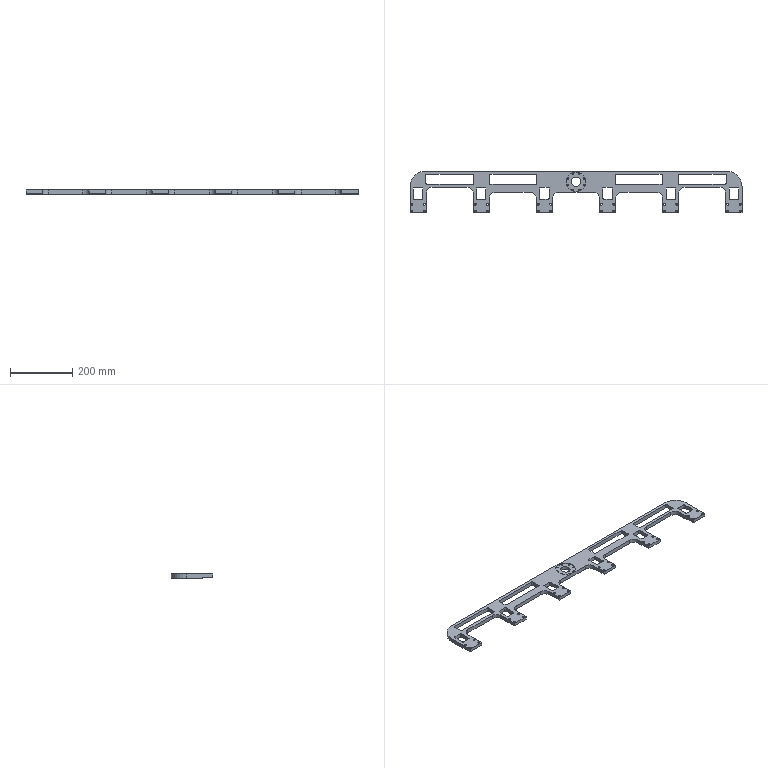NC program | NX | posted with a generic post | part box 1068 x 134 x 13 mm
Lines 1 to 1284 of 4175:
N10 G17 G21 G94 G90
(FLOOR_WALL_COPY_COPY , TOOL : D63)
N12 T01 M6
N14 G54
N16 G17 G0 G90 X572.5 Y-70.997 S6500 M3
N18 G43 Z30. H1
N20 Z4.
N22 G94 G1 Z1. F1500.
N24 X569.5
N26 X117.6
N28 Y-41.798
N30 X569.5
N32 Y-12.599
N34 X117.6
N36 Y16.601
N38 X569.5
N40 Y45.8
N42 X117.6
N44 Y74.999
N46 X569.5
N48 X572.5
N50 Z4.
N52 G0 Z30.
N54 Y-70.997
N56 Z3.
N58 G1 Z0.
N60 X569.5
N62 X117.6
N64 Y-41.798
N66 X569.5
N68 Y-12.599
N70 X117.6
N72 Y16.601
N74 X569.5
N76 Y45.8
N78 X117.6
N80 Y74.999
N82 X569.5
N84 X572.5
N86 Z3.
N88 G0 Z30.
N90 M5
(DRILLING_COPY_1_COPY , TOOL : D6A45)
N92 T07 M6
N94 G54
N96 G17 G0 G90 X284.8 Y-39.2 S5000 M3
N98 G43 Z30. H7
N100 G94 G81 G98 Z-1. F250. R3.
N102 Y-61.2
N104 X324.8
N106 Y-39.2
N108 X488.
N110 Y-61.2
N112 X528.
N114 Y-39.2
N116 G80
N118 G0 X528. Y-39.2 Z30.
N120 M5
(DRILLING_COPY_COPY_COPY_COPY , TOOL : 6.5ZT)
N122 T15 M6
N124 G54
N126 G17 G0 G90 X284.8 Y-39.2 S2000 M3
N128 G43 Z30. H15
N130 G94 G83 G98 Z-15.953 F250. Q2. R3.
N132 Y-61.2
N134 X324.8
N136 Y-39.2
N138 X488.
N140 Y-61.2
N142 X528.
N144 Y-39.2
N146 G80
N148 G0 X528. Y-39.2 Z30.
N150 M5
(ZLEVEL_PROFILE_COPY_3_COPY_1 , TOOL : D10)
N152 T10 M6
N154 G54
N156 G17 G0 G90 X115.002 Y75.6 S9500 M3
N158 G43 Z30. H10
N160 Z4.046
N162 G94 G1 Z-0.954 F1000.
N164 X116.734 Y72.6
N166 G3 X117.6 Y72.1 R1.
N168 G1 X484. F3500.
N170 G2 X539.1 Y17. R55.1
N172 G1 Y-67.
N174 G2 X534. Y-72.1 R5.1
N176 G1 X482.
N178 G2 X476.9 Y-67. R5.1
N180 G1 Y-5.
N182 G3 X462. Y9.9 R14.9
N184 G1 X350.8
N186 G3 X335.9 Y-5. R14.9
N188 G1 Y-67.
N190 G2 X330.8 Y-72.1 R5.1
N192 G1 X278.8
N194 G2 X273.7 Y-67. R5.1
N196 G1 Y-20.95
N198 G3 X258.8 Y-6.05 R14.9
N200 G1 X147.6
N202 G3 X132.7 Y-20.95 R14.9
N204 G1 Y-67.
N206 G2 X127.6 Y-72.1 R5.1
N208 G1 X117.6
N210 G3 X116.734 Y-72.6 R1.
N212 G1 X115.002 Y-75.6
N214 Z4.046
N216 G0 Z30.
N218 Z3.092
N220 G1 Z-1.908 F1000.
N222 X116.734 Y-72.6
N224 G2 X117.6 Y-72.1 R1.
N226 G1 X127.6 F3500.
N228 G3 X132.7 Y-67. R5.1
N230 G1 Y-20.95
N232 G2 X147.6 Y-6.05 R14.9
N234 G1 X258.8
N236 G2 X273.7 Y-20.95 R14.9
N238 G1 Y-67.
N240 G3 X278.8 Y-72.1 R5.1
N242 G1 X330.8
N244 G3 X335.9 Y-67. R5.1
N246 G1 Y-5.
N248 G2 X350.8 Y9.9 R14.9
N250 G1 X462.
N252 G2 X476.9 Y-5. R14.9
N254 G1 Y-67.
N256 G3 X482. Y-72.1 R5.1
N258 G1 X534.
N260 G3 X539.1 Y-67. R5.1
N262 G1 Y17.
N264 G3 X484. Y72.1 R55.1
N266 G1 X117.6
N268 G2 X116.734 Y72.6 R1.
N270 G1 X115.002 Y75.6
N272 Z3.092
N274 G0 Z30.
N276 Z2.138
N278 G1 Z-2.862 F1000.
N280 X116.734 Y72.6
N282 G3 X117.6 Y72.1 R1.
N284 G1 X484. F3500.
N286 G2 X539.1 Y17. R55.1
N288 G1 Y-67.
N290 G2 X534. Y-72.1 R5.1
N292 G1 X482.
N294 G2 X476.9 Y-67. R5.1
N296 G1 Y-5.
N298 G3 X462. Y9.9 R14.9
N300 G1 X350.8
N302 G3 X335.9 Y-5. R14.9
N304 G1 Y-67.
N306 G2 X330.8 Y-72.1 R5.1
N308 G1 X278.8
N310 G2 X273.7 Y-67. R5.1
N312 G1 Y-20.95
N314 G3 X258.8 Y-6.05 R14.9
N316 G1 X147.6
N318 G3 X132.7 Y-20.95 R14.9
N320 G1 Y-67.
N322 G2 X127.6 Y-72.1 R5.1
N324 G1 X117.6
N326 G3 X116.734 Y-72.6 R1.
N328 G1 X115.002 Y-75.6
N330 Z2.138
N332 G0 Z30.
N334 Z1.185
N336 G1 Z-3.815 F1000.
N338 X116.734 Y-72.6
N340 G2 X117.6 Y-72.1 R1.
N342 G1 X127.6 F3500.
N344 G3 X132.7 Y-67. R5.1
N346 G1 Y-20.95
N348 G2 X147.6 Y-6.05 R14.9
N350 G1 X258.8
N352 G2 X273.7 Y-20.95 R14.9
N354 G1 Y-67.
N356 G3 X278.8 Y-72.1 R5.1
N358 G1 X330.8
N360 G3 X335.9 Y-67. R5.1
N362 G1 Y-5.
N364 G2 X350.8 Y9.9 R14.9
N366 G1 X462.
N368 G2 X476.9 Y-5. R14.9
N370 G1 Y-67.
N372 G3 X482. Y-72.1 R5.1
N374 G1 X534.
N376 G3 X539.1 Y-67. R5.1
N378 G1 Y17.
N380 G3 X484. Y72.1 R55.1
N382 G1 X117.6
N384 G2 X116.734 Y72.6 R1.
N386 G1 X115.002 Y75.6
N388 Z1.185
N390 G0 Z30.
N392 Z0.231
N394 G1 Z-4.769 F1000.
N396 X116.734 Y72.6
N398 G3 X117.6 Y72.1 R1.
N400 G1 X484. F3500.
N402 G2 X539.1 Y17. R55.1
N404 G1 Y-67.
N406 G2 X534. Y-72.1 R5.1
N408 G1 X482.
N410 G2 X476.9 Y-67. R5.1
N412 G1 Y-5.
N414 G3 X462. Y9.9 R14.9
N416 G1 X350.8
N418 G3 X335.9 Y-5. R14.9
N420 G1 Y-67.
N422 G2 X330.8 Y-72.1 R5.1
N424 G1 X278.8
N426 G2 X273.7 Y-67. R5.1
N428 G1 Y-20.95
N430 G3 X258.8 Y-6.05 R14.9
N432 G1 X147.6
N434 G3 X132.7 Y-20.95 R14.9
N436 G1 Y-67.
N438 G2 X127.6 Y-72.1 R5.1
N440 G1 X117.6
N442 G3 X116.734 Y-72.6 R1.
N444 G1 X115.002 Y-75.6
N446 Z0.231
N448 G0 Z30.
N450 Z-0.723
N452 G1 Z-5.723 F1000.
N454 X116.734 Y-72.6
N456 G2 X117.6 Y-72.1 R1.
N458 G1 X127.6 F3500.
N460 G3 X132.7 Y-67. R5.1
N462 G1 Y-20.95
N464 G2 X147.6 Y-6.05 R14.9
N466 G1 X258.8
N468 G2 X273.7 Y-20.95 R14.9
N470 G1 Y-67.
N472 G3 X278.8 Y-72.1 R5.1
N474 G1 X330.8
N476 G3 X335.9 Y-67. R5.1
N478 G1 Y-5.
N480 G2 X350.8 Y9.9 R14.9
N482 G1 X462.
N484 G2 X476.9 Y-5. R14.9
N486 G1 Y-67.
N488 G3 X482. Y-72.1 R5.1
N490 G1 X534.
N492 G3 X539.1 Y-67. R5.1
N494 G1 Y17.
N496 G3 X484. Y72.1 R55.1
N498 G1 X117.6
N500 G2 X116.734 Y72.6 R1.
N502 G1 X115.002 Y75.6
N504 Z-0.723
N506 G0 Z30.
N508 Z-1.677
N510 G1 Z-6.677 F1000.
N512 X116.734 Y72.6
N514 G3 X117.6 Y72.1 R1.
N516 G1 X484. F3500.
N518 G2 X539.1 Y17. R55.1
N520 G1 Y-67.
N522 G2 X534. Y-72.1 R5.1
N524 G1 X482.
N526 G2 X476.9 Y-67. R5.1
N528 G1 Y-5.
N530 G3 X462. Y9.9 R14.9
N532 G1 X350.8
N534 G3 X335.9 Y-5. R14.9
N536 G1 Y-67.
N538 G2 X330.8 Y-72.1 R5.1
N540 G1 X278.8
N542 G2 X273.7 Y-67. R5.1
N544 G1 Y-20.95
N546 G3 X258.8 Y-6.05 R14.9
N548 G1 X147.6
N550 G3 X132.7 Y-20.95 R14.9
N552 G1 Y-67.
N554 G2 X127.6 Y-72.1 R5.1
N556 G1 X117.6
N558 G3 X116.734 Y-72.6 R1.
N560 G1 X115.002 Y-75.6
N562 Z-1.677
N564 G0 Z30.
N566 Z-2.631
N568 G1 Z-7.631 F1000.
N570 X116.734 Y-72.6
N572 G2 X117.6 Y-72.1 R1.
N574 G1 X127.6 F3500.
N576 G3 X132.7 Y-67. R5.1
N578 G1 Y-20.95
N580 G2 X147.6 Y-6.05 R14.9
N582 G1 X258.8
N584 G2 X273.7 Y-20.95 R14.9
N586 G1 Y-67.
N588 G3 X278.8 Y-72.1 R5.1
N590 G1 X330.8
N592 G3 X335.9 Y-67. R5.1
N594 G1 Y-5.
N596 G2 X350.8 Y9.9 R14.9
N598 G1 X462.
N600 G2 X476.9 Y-5. R14.9
N602 G1 Y-67.
N604 G3 X482. Y-72.1 R5.1
N606 G1 X534.
N608 G3 X539.1 Y-67. R5.1
N610 G1 Y17.
N612 G3 X484. Y72.1 R55.1
N614 G1 X117.6
N616 G2 X116.734 Y72.6 R1.
N618 G1 X115.002 Y75.6
N620 Z-2.631
N622 G0 Z30.
N624 Z-3.585
N626 G1 Z-8.585 F1000.
N628 X116.734 Y72.6
N630 G3 X117.6 Y72.1 R1.
N632 G1 X484. F3500.
N634 G2 X539.1 Y17. R55.1
N636 G1 Y-67.
N638 G2 X534. Y-72.1 R5.1
N640 G1 X482.
N642 G2 X476.9 Y-67. R5.1
N644 G1 Y-5.
N646 G3 X462. Y9.9 R14.9
N648 G1 X350.8
N650 G3 X335.9 Y-5. R14.9
N652 G1 Y-67.
N654 G2 X330.8 Y-72.1 R5.1
N656 G1 X278.8
N658 G2 X273.7 Y-67. R5.1
N660 G1 Y-20.95
N662 G3 X258.8 Y-6.05 R14.9
N664 G1 X147.6
N666 G3 X132.7 Y-20.95 R14.9
N668 G1 Y-67.
N670 G2 X127.6 Y-72.1 R5.1
N672 G1 X117.6
N674 G3 X116.734 Y-72.6 R1.
N676 G1 X115.002 Y-75.6
N678 Z-3.585
N680 G0 Z30.
N682 Z-4.538
N684 G1 Z-9.538 F1000.
N686 X116.734 Y-72.6
N688 G2 X117.6 Y-72.1 R1.
N690 G1 X127.6 F3500.
N692 G3 X132.7 Y-67. R5.1
N694 G1 Y-20.95
N696 G2 X147.6 Y-6.05 R14.9
N698 G1 X258.8
N700 G2 X273.7 Y-20.95 R14.9
N702 G1 Y-67.
N704 G3 X278.8 Y-72.1 R5.1
N706 G1 X330.8
N708 G3 X335.9 Y-67. R5.1
N710 G1 Y-5.
N712 G2 X350.8 Y9.9 R14.9
N714 G1 X462.
N716 G2 X476.9 Y-5. R14.9
N718 G1 Y-67.
N720 G3 X482. Y-72.1 R5.1
N722 G1 X534.
N724 G3 X539.1 Y-67. R5.1
N726 G1 Y17.
N728 G3 X484. Y72.1 R55.1
N730 G1 X117.6
N732 G2 X116.734 Y72.6 R1.
N734 G1 X115.002 Y75.6
N736 Z-4.538
N738 G0 Z30.
N740 Z-5.492
N742 G1 Z-10.492 F1000.
N744 X116.734 Y72.6
N746 G3 X117.6 Y72.1 R1.
N748 G1 X484. F3500.
N750 G2 X539.1 Y17. R55.1
N752 G1 Y-67.
N754 G2 X534. Y-72.1 R5.1
N756 G1 X482.
N758 G2 X476.9 Y-67. R5.1
N760 G1 Y-5.
N762 G3 X462. Y9.9 R14.9
N764 G1 X350.8
N766 G3 X335.9 Y-5. R14.9
N768 G1 Y-67.
N770 G2 X330.8 Y-72.1 R5.1
N772 G1 X278.8
N774 G2 X273.7 Y-67. R5.1
N776 G1 Y-20.95
N778 G3 X258.8 Y-6.05 R14.9
N780 G1 X147.6
N782 G3 X132.7 Y-20.95 R14.9
N784 G1 Y-67.
N786 G2 X127.6 Y-72.1 R5.1
N788 G1 X117.6
N790 G3 X116.734 Y-72.6 R1.
N792 G1 X115.002 Y-75.6
N794 Z-5.492
N796 G0 Z30.
N798 Z-6.446
N800 G1 Z-11.446 F1000.
N802 X116.734 Y-72.6
N804 G2 X117.6 Y-72.1 R1.
N806 G1 X127.6 F3500.
N808 G3 X132.7 Y-67. R5.1
N810 G1 Y-20.95
N812 G2 X147.6 Y-6.05 R14.9
N814 G1 X258.8
N816 G2 X273.7 Y-20.95 R14.9
N818 G1 Y-67.
N820 G3 X278.8 Y-72.1 R5.1
N822 G1 X330.8
N824 G3 X335.9 Y-67. R5.1
N826 G1 Y-5.
N828 G2 X350.8 Y9.9 R14.9
N830 G1 X462.
N832 G2 X476.9 Y-5. R14.9
N834 G1 Y-67.
N836 G3 X482. Y-72.1 R5.1
N838 G1 X534.
N840 G3 X539.1 Y-67. R5.1
N842 G1 Y17.
N844 G3 X484. Y72.1 R55.1
N846 G1 X117.6
N848 G2 X116.734 Y72.6 R1.
N850 G1 X115.002 Y75.6
N852 Z-6.446
N854 G0 Z30.
N856 Z-7.4
N858 G1 Z-12.4 F1000.
N860 X116.734 Y72.6
N862 G3 X117.6 Y72.1 R1.
N864 G1 X484. F3500.
N866 G2 X539.1 Y17. R55.1
N868 G1 Y-67.
N870 G2 X534. Y-72.1 R5.1
N872 G1 X482.
N874 G2 X476.9 Y-67. R5.1
N876 G1 Y-5.
N878 G3 X462. Y9.9 R14.9
N880 G1 X350.8
N882 G3 X335.9 Y-5. R14.9
N884 G1 Y-67.
N886 G2 X330.8 Y-72.1 R5.1
N888 G1 X278.8
N890 G2 X273.7 Y-67. R5.1
N892 G1 Y-20.95
N894 G3 X258.8 Y-6.05 R14.9
N896 G1 X147.6
N898 G3 X132.7 Y-20.95 R14.9
N900 G1 Y-67.
N902 G2 X127.6 Y-72.1 R5.1
N904 G1 X117.6
N906 G3 X116.734 Y-72.6 R1.
N908 G1 X115.002 Y-75.6
N910 Z-7.4
N912 G0 Z30.
(ZLEVEL_PROFILE_COPY_2_COPY_COPY , TOOL : D10)
N914 X453.956 Y51.9
N916 Z1.5
N918 G1 X406.4 Z-0.992 F1000.
N920 X334.935 F3500.
N922 X334.9 Y51.902
N924 Y30.1
N926 X477.9
N928 Y51.902
N930 X477.86 Y51.9
N932 X406.4
N934 X349.551 Z-1.985
N936 X334.935
N938 X334.9 Y51.902
N940 Y30.1
N942 X477.9
N944 Y51.902
N946 X477.86 Y51.9
N948 X406.4
N950 X349.551 Z-2.977
N952 X334.935
N954 X334.9 Y51.902
N956 Y30.1
N958 X477.9
N960 Y51.902
N962 X477.86 Y51.9
N964 X406.4
N966 X349.551 Z-3.969
N968 X334.935
N970 X334.9 Y51.902
N972 Y30.1
N974 X477.9
N976 Y51.902
N978 X477.86 Y51.9
N980 X406.4
N982 X349.551 Z-4.962
N984 X334.935
N986 X334.9 Y51.902
N988 Y30.1
N990 X477.9
N992 Y51.902
N994 X477.86 Y51.9
N996 X406.4
N998 X349.551 Z-5.954
N1000 X334.935
N1002 X334.9 Y51.902
N1004 Y30.1
N1006 X477.9
N1008 Y51.902
N1010 X477.86 Y51.9
N1012 X406.4
N1014 X349.551 Z-6.946
N1016 X334.935
N1018 X334.9 Y51.902
N1020 Y30.1
N1022 X477.9
N1024 Y51.902
N1026 X477.86 Y51.9
N1028 X406.4
N1030 X349.551 Z-7.938
N1032 X334.935
N1034 X334.9 Y51.902
N1036 Y30.1
N1038 X477.9
N1040 Y51.902
N1042 X477.86 Y51.9
N1044 X406.4
N1046 X349.551 Z-8.931
N1048 X334.935
N1050 X334.9 Y51.902
N1052 Y30.1
N1054 X477.9
N1056 Y51.902
N1058 X477.86 Y51.9
N1060 X406.4
N1062 X349.551 Z-9.923
N1064 X334.935
N1066 X334.9 Y51.902
N1068 Y30.1
N1070 X477.9
N1072 Y51.902
N1074 X477.86 Y51.9
N1076 X406.4
N1078 X349.551 Z-10.915
N1080 X334.935
N1082 X334.9 Y51.902
N1084 Y30.1
N1086 X477.9
N1088 Y51.902
N1090 X477.86 Y51.9
N1092 X406.4
N1094 X349.551 Z-11.908
N1096 X334.935
N1098 X334.9 Y51.902
N1100 Y30.1
N1102 X477.9
N1104 Y51.902
N1106 X477.86 Y51.9
N1108 X406.4
N1110 X349.551 Z-12.9
N1112 X334.935
N1114 X334.9 Y51.902
N1116 Y30.1
N1118 X477.9
N1120 Y51.902
N1122 X477.86 Y51.9
N1124 X349.551
N1126 Z-11.4
N1128 G0 Z30.
N1130 X250.756
N1132 Z1.5
N1134 G1 X203.2 Z-0.992 F1000.
N1136 X131.735 F3500.
N1138 X131.7 Y51.902
N1140 Y30.1
N1142 X274.7
N1144 Y51.902
N1146 X274.66 Y51.9
N1148 X203.2
N1150 X146.351 Z-1.985
N1152 X131.735
N1154 X131.7 Y51.902
N1156 Y30.1
N1158 X274.7
N1160 Y51.902
N1162 X274.66 Y51.9
N1164 X203.2
N1166 X146.351 Z-2.977
N1168 X131.735
N1170 X131.7 Y51.902
N1172 Y30.1
N1174 X274.7
N1176 Y51.902
N1178 X274.66 Y51.9
N1180 X203.2
N1182 X146.351 Z-3.969
N1184 X131.735
N1186 X131.7 Y51.902
N1188 Y30.1
N1190 X274.7
N1192 Y51.902
N1194 X274.66 Y51.9
N1196 X203.2
N1198 X146.351 Z-4.962
N1200 X131.735
N1202 X131.7 Y51.902
N1204 Y30.1
N1206 X274.7
N1208 Y51.902
N1210 X274.66 Y51.9
N1212 X203.2
N1214 X146.351 Z-5.954
N1216 X131.735
N1218 X131.7 Y51.902
N1220 Y30.1
N1222 X274.7
N1224 Y51.902
N1226 X274.66 Y51.9
N1228 X203.2
N1230 X146.351 Z-6.946
N1232 X131.735
N1234 X131.7 Y51.902
N1236 Y30.1
N1238 X274.7
N1240 Y51.902
N1242 X274.66 Y51.9
N1244 X203.2
N1246 X146.351 Z-7.938
N1248 X131.735
N1250 X131.7 Y51.902
N1252 Y30.1
N1254 X274.7
N1256 Y51.902
N1258 X274.66 Y51.9
N1260 X203.2
N1262 X146.351 Z-8.931
N1264 X131.735
N1266 X131.7 Y51.902
N1268 Y30.1
N1270 X274.7
N1272 Y51.902
N1274 X274.66 Y51.9
N1276 X203.2
N1278 X146.351 Z-9.923
N1280 X131.735
N1282 X131.7 Y51.902
N1284 Y30.1
N1286 X274.7
N1288 Y51.902
N1290 X274.66 Y51.9
N1292 X203.2
N1294 X146.351 Z-10.915
N1296 X131.735
N1298 X131.7 Y51.902
N1300 Y30.1
N1302 X274.7
N1304 Y51.902
N1306 X274.66 Y51.9
N1308 X203.2
N1310 X146.351 Z-11.908
N1312 X131.735
N1314 X131.7 Y51.902
N1316 Y30.1
N1318 X274.7
N1320 Y51.902
N1322 X274.66 Y51.9
N1324 X203.2
N1326 X146.351 Z-12.9
N1328 X131.735
N1330 X131.7 Y51.902
N1332 Y30.1
N1334 X274.7
N1336 Y51.902
N1338 X274.66 Y51.9
N1340 X146.351
N1342 Z-11.4
N1344 G0 Z30.
N1346 X498.1 Y-6.045
N1348 Z1.5
N1350 G1 Y-18.9 Z0.826 F1000.
N1352 X517.9 Z-0.211
N1354 Y-3.999 Z-0.992
N1356 Y10.903 F3500.
N1358 X517.852 Y10.9
N1360 X498.147
N1362 X498.1 Y10.902
N1364 Y-18.9
N1366 X517.9
N1368 Y-3.999
N1370 Y10.658 Z-1.248
N1372 Y10.9 Z-1.252
N1374 X517.701 Z-1.256
N1376 X498.159 Z-1.597
N1378 X498.1 Z-1.598
N1380 Y10.517 Z-1.605
N1382 Y-11.246 Z-1.985
N1384 Y-18.9
N1386 X517.9
N1388 Y-3.999
N1390 Y10.658 Z-2.24
N1392 Y10.9 Z-2.245
N1394 X517.701 Z-2.248
N1396 X498.159 Z-2.589
N1398 X498.1 Z-2.59
N1400 Y10.517 Z-2.597
N1402 Y-11.246 Z-2.977
N1404 Y-18.9
N1406 X517.9
N1408 Y-3.999
N1410 Y10.658 Z-3.233
N1412 Y10.9 Z-3.237
N1414 X517.701 Z-3.241
N1416 X498.159 Z-3.582
N1418 X498.1 Z-3.583
N1420 Y10.517 Z-3.589
N1422 Y-11.246 Z-3.969
N1424 Y-18.9
N1426 X517.9
N1428 Y-3.999
N1430 Y10.658 Z-4.225
N1432 Y10.9 Z-4.229
N1434 X517.701 Z-4.233
N1436 X498.159 Z-4.574
N1438 X498.1 Z-4.575
N1440 Y10.517 Z-4.582
N1442 Y-11.246 Z-4.962
N1444 Y-18.9
N1446 X517.9
N1448 Y-3.999
N1450 Y10.658 Z-5.217
N1452 Y10.9 Z-5.222
N1454 X517.701 Z-5.225
N1456 X498.159 Z-5.566
N1458 X498.1 Z-5.567
N1460 Y10.517 Z-5.574
N1462 Y-11.246 Z-5.954
N1464 Y-18.9
N1466 X517.9
N1468 Y-3.999
N1470 Y10.658 Z-6.21
N1472 Y10.9 Z-6.214
N1474 X517.701 Z-6.217
N1476 X498.159 Z-6.559
N1478 X498.1 Z-6.56
N1480 Y10.517 Z-6.566
N1482 Y-11.246 Z-6.946
N1484 Y-18.9
N1486 X517.9
N1488 Y-3.999
N1490 Y10.658 Z-7.202
N1492 Y10.9 Z-7.206
N1494 X517.701 Z-7.21
N1496 X498.159 Z-7.551
N1498 X498.1 Z-7.552
N1500 Y10.517 Z-7.559
N1502 Y-11.246 Z-7.938
N1504 Y-18.9
N1506 X517.9
N1508 Y-3.999
N1510 Y10.658 Z-8.194
N1512 Y10.9 Z-8.199
N1514 X517.701 Z-8.202
N1516 X498.159 Z-8.543
N1518 X498.1 Z-8.544
N1520 Y10.517 Z-8.551
N1522 Y-11.246 Z-8.931
N1524 Y-18.9
N1526 X517.9
N1528 Y-3.999
N1530 Y10.658 Z-9.187
N1532 Y10.9 Z-9.191
N1534 X517.701 Z-9.194
N1536 X498.159 Z-9.535
N1538 X498.1 Z-9.536
N1540 Y10.517 Z-9.543
N1542 Y-11.246 Z-9.923
N1544 Y-18.9
N1546 X517.9
N1548 Y-3.999
N1550 Y10.658 Z-10.179
N1552 Y10.9 Z-10.183
N1554 X517.701 Z-10.187
N1556 X498.159 Z-10.528
N1558 X498.1 Z-10.529
N1560 Y10.517 Z-10.536
N1562 Y-11.246 Z-10.915
N1564 Y-18.9
N1566 X517.9
N1568 Y-3.999
N1570 Y10.658 Z-11.171
N1572 Y10.9 Z-11.175
N1574 X517.701 Z-11.179
N1576 X498.159 Z-11.52
N1578 X498.1 Z-11.521
N1580 Y10.517 Z-11.528
N1582 Y-11.246 Z-11.908
N1584 Y-18.9
N1586 X517.9
N1588 Y-3.999
N1590 Y10.658 Z-12.164
N1592 Y10.9 Z-12.168
N1594 X517.701 Z-12.171
N1596 X498.159 Z-12.512
N1598 X498.1 Z-12.513
N1600 Y10.517 Z-12.52
N1602 Y-11.246 Z-12.9
N1604 Y-18.9
N1606 X517.9
N1608 Y10.903
N1610 X517.852 Y10.9
N1612 X498.147
N1614 X498.1 Y10.902
N1616 Y-11.246
N1618 Z-11.4
N1620 G0 Z30.
N1622 X294.9 Y-6.044
N1624 Z1.5
N1626 G1 Y-18.9 Z0.826 F1000.
N1628 X314.7 Z-0.211
N1630 Y-4. Z-0.992
N1632 Y10.9 F3500.
N1634 X294.942
N1636 X294.9 Y10.902
N1638 Y-18.9
N1640 X314.7
N1642 Y-4.
N1644 Y10.9 Z-1.252
N1646 X294.957 Z-1.597
N1648 X294.9 Z-1.598
N1650 Y10.515 Z-1.605
N1652 Y-11.248 Z-1.985
N1654 Y-18.9
N1656 X314.7
N1658 Y-4.
N1660 Y10.9 Z-2.245
N1662 X294.957 Z-2.589
N1664 X294.9 Z-2.59
N1666 Y10.515 Z-2.597
N1668 Y-11.248 Z-2.977
N1670 Y-18.9
N1672 X314.7
N1674 Y-4.
N1676 Y10.9 Z-3.237
N1678 X294.957 Z-3.582
N1680 X294.9 Z-3.583
N1682 Y10.515 Z-3.589
N1684 Y-11.248 Z-3.969
N1686 Y-18.9
N1688 X314.7
N1690 Y-4.
N1692 Y10.9 Z-4.229
N1694 X294.957 Z-4.574
N1696 X294.9 Z-4.575
N1698 Y10.515 Z-4.582
N1700 Y-11.248 Z-4.962
N1702 Y-18.9
N1704 X314.7
N1706 Y-4.
N1708 Y10.9 Z-5.222
N1710 X294.957 Z-5.566
N1712 X294.9 Z-5.567
N1714 Y10.515 Z-5.574
N1716 Y-11.248 Z-5.954
N1718 Y-18.9
N1720 X314.7
N1722 Y-4.
N1724 Y10.9 Z-6.214
N1726 X294.957 Z-6.559
N1728 X294.9 Z-6.56
N1730 Y10.515 Z-6.566
N1732 Y-11.248 Z-6.946
N1734 Y-18.9
N1736 X314.7
N1738 Y-4.
N1740 Y10.9 Z-7.206
N1742 X294.957 Z-7.551
N1744 X294.9 Z-7.552
N1746 Y10.515 Z-7.559
N1748 Y-11.248 Z-7.938
N1750 Y-18.9
N1752 X314.7
N1754 Y-4.
N1756 Y10.9 Z-8.199
N1758 X294.957 Z-8.543
N1760 X294.9 Z-8.544
N1762 Y10.515 Z-8.551
N1764 Y-11.248 Z-8.931
N1766 Y-18.9
N1768 X314.7
N1770 Y-4.
N1772 Y10.9 Z-9.191
N1774 X294.957 Z-9.535
N1776 X294.9 Z-9.536
N1778 Y10.515 Z-9.543
N1780 Y-11.248 Z-9.923
N1782 Y-18.9
N1784 X314.7
N1786 Y-4.
N1788 Y10.9 Z-10.183
N1790 X294.957 Z-10.528
N1792 X294.9 Z-10.529
N1794 Y10.514 Z-10.536
N1796 Y-11.248 Z-10.915
N1798 Y-18.9
N1800 X314.7
N1802 Y-4.
N1804 Y10.9 Z-11.175
N1806 X294.957 Z-11.52
N1808 X294.9 Z-11.521
N1810 Y10.514 Z-11.528
N1812 Y-11.248 Z-11.908
N1814 Y-18.9
N1816 X314.7
N1818 Y-4.
N1820 Y10.9 Z-12.168
N1822 X294.957 Z-12.512
N1824 X294.9 Z-12.513
N1826 Y10.514 Z-12.52
N1828 Y-11.248 Z-12.9
N1830 Y-18.9
N1832 X314.7
N1834 Y10.9
N1836 X294.942
N1838 X294.9 Y10.901
N1840 Y-11.248
N1842 Z-11.4
N1844 G0 Z30.
(ZLEVEL_PROFILE_COPY_COPY_1_COPY , TOOL : D10)
N1846 X254.551 Y30.
N1848 Z1.
N1850 G1 X274.8 Z-2.57 F1000.
N1852 Y52.002 Z-6.45
N1854 X274.754 Y52. F1500.
N1856 X131.645
N1858 X131.6 Y52.002
N1860 Y30.
N1862 X274.8
N1864 Y52.002
N1866 X274.577 Y52. Z-6.456
N1868 X131.793 Z-10.172
N1870 X131.6 Y51.972 Z-10.178
N1872 Y30.074 Z-10.748
N1874 X131.749 Y30. Z-10.754
N1876 X214.201 Z-12.9
N1878 X274.8
N1880 Y52.002
N1882 X274.754 Y52.
N1884 X131.645
N1886 X131.6 Y52.002
N1888 Y30.
N1890 X214.201
N1892 Z-11.9
N1894 G0 Z30.
N1896 X314.8 Y-11.249
N1898 Z1.
N1900 G1 Y11.002 Z-2.923 F1000.
N1902 X314.754 Y11. Z-2.932
N1904 X294.835 Z-6.444
N1906 X294.8 Y11.003 Z-6.45
N1908 Y-19. F1500.
N1910 X314.8
N1912 Y11.002
N1914 X314.754 Y11.
N1916 X294.835
N1918 X294.8 Y11.003
N1920 Y10.779 Z-6.469
N1922 Y-18.91 Z-9.022
N1924 X294.933 Y-19. Z-9.042
N1926 X314.8 Z-10.75
N1928 Y-18.777 Z-10.769
N1930 Y6.001 Z-12.9
N1932 Y11.002
N1934 X314.754 Y11.
N1936 X294.835
N1938 X294.8 Y11.002
N1940 Y-19.
N1942 X314.8
N1944 Y6.001
N1946 Z-11.9
N1948 G0 Z30.
N1950 X457.751 Y30.
N1952 Z1.
N1954 G1 X478. Z-2.57 F1000.
N1956 Y52.002 Z-6.45
N1958 X477.966 Y52. F1500.
N1960 X334.846
N1962 X334.8 Y52.002
N1964 Y30.
N1966 X478.
N1968 Y52.002
N1970 X477.777 Y52. Z-6.456
N1972 X334.994 Z-10.172
N1974 X334.8 Y51.972 Z-10.178
N1976 Y30.074 Z-10.748
N1978 X334.949 Y30. Z-10.754
N1980 X417.401 Z-12.9
N1982 X478.
N1984 Y52.002
N1986 X477.966 Y52.
N1988 X334.846
N1990 X334.8 Y52.002
N1992 Y30.
N1994 X417.401
N1996 Z-11.9
N1998 G0 Z30.
N2000 X498. Y3.251
N2002 Z1.
N2004 G1 Y-19. Z-2.923 F1000.
N2006 X518. Z-6.45
N2008 Y11.002 F1500.
N2010 X517.955 Y11.
N2012 X498.037
N2014 X498. Y11.002
N2016 Y-19.
N2018 X518.
N2020 Y10.912 Z-9.022
N2022 X517.867 Y11. Z-9.042
N2024 X498.223 Z-10.731
N2026 X498. Y11.002 Z-10.75
N2028 Y-13.999 Z-12.9
N2030 Y-19.
N2032 X518.
N2034 Y11.002
N2036 X517.955 Y11.
N2038 X498.037
N2040 X498. Y11.002
N2042 Y-13.999
N2044 Z-11.9
N2046 G0 Z30.
(FLOOR_WALL_1_COPY_1_COPY , TOOL : D10)
N2048 X306.243 Y-73.5
N2050 Z0.533
N2052 G1 Z-0.967 F1000.
N2054 X305.666 Y-72.5
N2056 G3 X304.8 Y-72. R1.
N2058 G1 X273.8 F3000.
N2060 Y-38.5
N2062 X335.8
N2064 Y-72.
N2066 X304.8
N2068 Y-66.
N2070 X279.8
N2072 Y-44.5
N2074 X329.8
N2076 Y-66.
N2078 X304.8
N2080 Y-60.
N2082 X285.8
N2084 Y-50.5
N2086 X323.8
N2088 Y-60.
N2090 X304.8
N2092 Y-55.5
N2094 X290.3
N2096 Y-55.
N2098 X319.3
N2100 Y-55.5
N2102 X304.8
N2104 G3 X303.934 Y-56. R1.
N2106 G1 Z0.533
N2108 G0 X306.243 Y-73.5 Z-0.433
N2110 G1 Z-1.933 F1000.
N2112 X305.666 Y-72.5
N2114 G3 X304.8 Y-72. R1.
N2116 G1 X273.8 F3000.
N2118 Y-38.5
N2120 X335.8
N2122 Y-72.
N2124 X304.8
N2126 Y-66.
N2128 X279.8
N2130 Y-44.5
N2132 X329.8
N2134 Y-66.
N2136 X304.8
N2138 Y-60.
N2140 X285.8
N2142 Y-50.5
N2144 X323.8
N2146 Y-60.
N2148 X304.8
N2150 Y-55.5
N2152 X290.3
N2154 Y-55.
N2156 X319.3
N2158 Y-55.5
N2160 X304.8
N2162 G3 X303.934 Y-56. R1.
N2164 G1 Z-0.433
N2166 G0 X306.243 Y-73.5 Z-1.4
N2168 G1 Z-2.9 F1000.
N2170 X305.666 Y-72.5
N2172 G3 X304.8 Y-72. R1.
N2174 G1 X273.8 F3000.
N2176 Y-38.5
N2178 X335.8
N2180 Y-72.
N2182 X304.8
N2184 Y-66.
N2186 X279.8
N2188 Y-44.5
N2190 X329.8
N2192 Y-66.
N2194 X304.8
N2196 Y-60.
N2198 X285.8
N2200 Y-50.5
N2202 X323.8
N2204 Y-60.
N2206 X304.8
N2208 Y-55.5
N2210 X290.3
N2212 Y-55.
N2214 X319.3
N2216 Y-55.5
N2218 X304.8
N2220 G3 X303.934 Y-56. R1.
N2222 G1 Z-1.4
N2224 G0 Z30.
N2226 X509.443 Y-73.5
N2228 Z0.533
N2230 G1 Z-0.967 F1000.
N2232 X508.866 Y-72.5
N2234 G3 X508. Y-72. R1.
N2236 G1 X477. F3000.
N2238 Y-38.5
N2240 X539.
N2242 Y-72.
N2244 X508.
N2246 Y-66.
N2248 X483.
N2250 Y-44.5
N2252 X533.
N2254 Y-66.
N2256 X508.
N2258 Y-60.
N2260 X489.
N2262 Y-50.5
N2264 X527.
N2266 Y-60.
N2268 X508.
N2270 Y-55.5
N2272 X493.5
N2274 Y-55.
N2276 X522.5
N2278 Y-55.5
N2280 X508.
N2282 G3 X507.134 Y-56. R1.
N2284 G1 Z0.533
N2286 G0 X509.443 Y-73.5 Z-0.433
N2288 G1 Z-1.933 F1000.
N2290 X508.866 Y-72.5
N2292 G3 X508. Y-72. R1.
N2294 G1 X477. F3000.
N2296 Y-38.5
N2298 X539.
N2300 Y-72.
N2302 X508.
N2304 Y-66.
N2306 X483.
N2308 Y-44.5
N2310 X533.
N2312 Y-66.
N2314 X508.
N2316 Y-60.
N2318 X489.
N2320 Y-50.5
N2322 X527.
N2324 Y-60.
N2326 X508.
N2328 Y-55.5
N2330 X493.5
N2332 Y-55.
N2334 X522.5
N2336 Y-55.5
N2338 X508.
N2340 G3 X507.134 Y-56. R1.
N2342 G1 Z-0.433
N2344 G0 X509.443 Y-73.5 Z-1.4
N2346 G1 Z-2.9 F1000.
N2348 X508.866 Y-72.5
N2350 G3 X508. Y-72. R1.
N2352 G1 X477. F3000.
N2354 Y-38.5
N2356 X539.
N2358 Y-72.
N2360 X508.
N2362 Y-66.
N2364 X483.
N2366 Y-44.5
N2368 X533.
N2370 Y-66.
N2372 X508.
N2374 Y-60.
N2376 X489.
N2378 Y-50.5
N2380 X527.
N2382 Y-60.
N2384 X508.
N2386 Y-55.5
N2388 X493.5
N2390 Y-55.
N2392 X522.5
N2394 Y-55.5
N2396 X508.
N2398 G3 X507.134 Y-56. R1.
N2400 G1 Z-1.4
N2402 G0 Z30.
(FLOOR_WALL_1_COPY_COPY_COPY , TOOL : D10)
N2404 X278.303 Y-72.866
N2406 Z-1.5
N2408 G1 Z-3. F1000.
N2410 G3 X278.803 Y-72. R1.
N2412 G1 Y-38.9 F1500.
N2414 X284.803
N2416 Y-72.
N2418 X290.802
N2420 Y-38.9
N2422 X296.802
N2424 Y-72.
N2426 X302.801
N2428 Y-38.9
N2430 X308.801
N2432 Y-72.
N2434 X314.801
N2436 Y-38.9
N2438 X320.8
N2440 Y-72.
N2442 X326.8
N2444 Y-38.9
N2446 G3 X325.934 Y-39.4 R1.
N2448 G1 Z-1.5
N2450 G0 X336.666 Y-38.9
N2452 G1 Z-3. F1000.
N2454 G3 X335.8 Y-38.4 R1.
N2456 G1 X273.8 F1500.
N2458 G3 X272.934 Y-38.9 R1.
N2460 G1 Z-1.5
N2462 G0 Z30.
N2464 X481.503 Y-72.866
N2466 Z-1.5
N2468 G1 Z-3. F1000.
N2470 G3 X482.003 Y-72. R1.
N2472 G1 Y-38.9 F1500.
N2474 X488.003
N2476 Y-72.
N2478 X494.002
N2480 Y-38.9
N2482 X500.002
N2484 Y-72.
N2486 X506.001
N2488 Y-38.9
N2490 X512.001
N2492 Y-72.
N2494 X518.001
N2496 Y-38.9
N2498 X524.
N2500 Y-72.
N2502 X530.
N2504 Y-38.9
N2506 G3 X529.134 Y-39.4 R1.
N2508 G1 Z-1.5
N2510 G0 X539.866 Y-38.9
N2512 G1 Z-3. F1000.
N2514 G3 X539. Y-38.4 R1.
N2516 G1 X477. F1500.
N2518 G3 X476.134 Y-38.9 R1.
N2520 G1 Z-1.5
N2522 G0 Z30.
N2524 M5